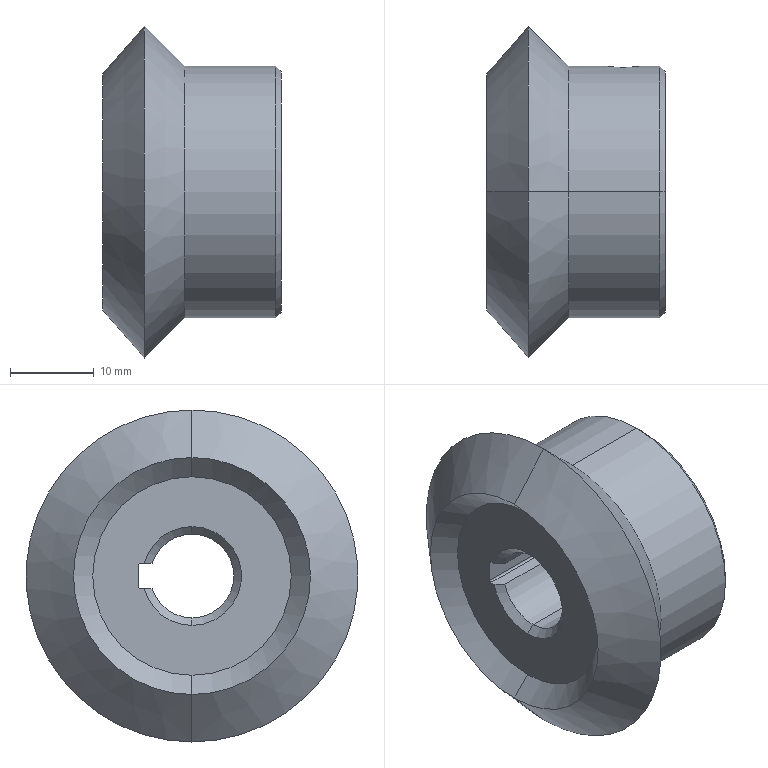Part | SolidWorks | features RefAxis 12, 3DProfileFeature 4, RevCut 2, ICE 1, Revolution 1 | 1 solid | 35 faces | box 21.26 x 39.62 x 39.62 mm | volume 14366 mm3 | cone 16 | cylinder 11 | plane 8 | commonest cylinder face diameters 0.4 x4 10 x3 3.242 x2 30 x2
STEP:
#1=CARTESIAN_POINT('',(-5.615,4.77,-1.5));
#2=VERTEX_POINT('',#1);
#3=CARTESIAN_POINT('',(-5.,4.73,-1.621));
#4=VERTEX_POINT('',#3);
#5=CARTESIAN_POINT('',(-5.615,4.77,-1.5));
#6=CARTESIAN_POINT('',(-5.518,4.757,-1.54));
#7=CARTESIAN_POINT('',(-5.418,4.747,-1.57));
#8=CARTESIAN_POINT('',(-5.211,4.734,-1.611));
#9=CARTESIAN_POINT('',(-5.105,4.73,-1.621));
#10=CARTESIAN_POINT('',(-5.,4.73,-1.621));
#11=B_SPLINE_CURVE_WITH_KNOTS('',3,(#5,#6,#7,#8,#9,#10),.UNSPECIFIED.,.F.,.F.,(4,2,4),(0.004473,0.004788,0.005103),.UNSPECIFIED.);
#12=EDGE_CURVE('',#2,#4,#11,.T.);
#13=ORIENTED_EDGE('',*,*,#12,.T.);
#14=CARTESIAN_POINT('',(-5.,14.621,-1.621));
#15=VERTEX_POINT('',#14);
#16=CARTESIAN_POINT('',(-5.,4.583,-1.621));
#17=DIRECTION('',(0.,1.,0.));
#18=VECTOR('',#17,1000.);
#19=LINE('',#16,#18);
#20=EDGE_CURVE('',#4,#15,#19,.T.);
#21=ORIENTED_EDGE('',*,*,#20,.T.);
#22=CARTESIAN_POINT('',(-5.,14.621,1.621));
#23=VERTEX_POINT('',#22);
#24=CARTESIAN_POINT('',(-5.,14.621,0.));
#25=DIRECTION('',(0.,1.,0.));
#26=DIRECTION('',(0.,0.,1.));
#27=AXIS2_PLACEMENT_3D('',#24,#25,#26);
#28=CIRCLE('',#27,1.621);
#29=EDGE_CURVE('',#15,#23,#28,.T.);
#30=ORIENTED_EDGE('',*,*,#29,.T.);
#31=CARTESIAN_POINT('',(-5.,4.73,1.621));
#32=VERTEX_POINT('',#31);
#33=CARTESIAN_POINT('',(-5.,4.583,1.621));
#34=DIRECTION('',(0.,1.,0.));
#35=VECTOR('',#34,1000.);
#36=LINE('',#33,#35);
#37=EDGE_CURVE('',#32,#23,#36,.T.);
#38=ORIENTED_EDGE('',*,*,#37,.F.);
#39=CARTESIAN_POINT('',(-5.615,4.77,1.5));
#40=VERTEX_POINT('',#39);
#41=CARTESIAN_POINT('',(-5.,4.73,1.621));
#42=CARTESIAN_POINT('',(-5.106,4.73,1.621));
#43=CARTESIAN_POINT('',(-5.211,4.734,1.611));
#44=CARTESIAN_POINT('',(-5.416,4.747,1.57));
#45=CARTESIAN_POINT('',(-5.518,4.757,1.54));
#46=CARTESIAN_POINT('',(-5.615,4.77,1.5));
#47=B_SPLINE_CURVE_WITH_KNOTS('',3,(#41,#42,#43,#44,#45,#46),.UNSPECIFIED.,.F.,.F.,(4,2,4),(0.,0.0003142,0.0006283),.UNSPECIFIED.);
#48=EDGE_CURVE('',#32,#40,#47,.T.);
#49=ORIENTED_EDGE('',*,*,#48,.T.);
#50=CARTESIAN_POINT('',(-5.615,6.2,1.5));
#51=VERTEX_POINT('',#50);
#52=CARTESIAN_POINT('',(-5.615,4.583,1.5));
#53=DIRECTION('',(0.,-1.,0.));
#54=VECTOR('',#53,1000.);
#55=LINE('',#52,#54);
#56=EDGE_CURVE('',#51,#40,#55,.T.);
#57=ORIENTED_EDGE('',*,*,#56,.F.);
#58=CARTESIAN_POINT('',(-5.968,6.4,1.3));
#59=VERTEX_POINT('',#58);
#60=CARTESIAN_POINT('',(-5.968,6.4,1.3));
#61=CARTESIAN_POINT('',(-5.903,6.4,1.349));
#62=CARTESIAN_POINT('',(-5.836,6.384,1.391));
#63=CARTESIAN_POINT('',(-5.736,6.34,1.445));
#64=CARTESIAN_POINT('',(-5.704,6.322,1.461));
#65=CARTESIAN_POINT('',(-5.659,6.286,1.481));
#66=CARTESIAN_POINT('',(-5.645,6.272,1.487));
#67=CARTESIAN_POINT('',(-5.623,6.24,1.497));
#68=CARTESIAN_POINT('',(-5.615,6.221,1.5));
#69=CARTESIAN_POINT('',(-5.615,6.2,1.5));
#70=B_SPLINE_CURVE_WITH_KNOTS('',3,(#60,#61,#62,#63,#64,#65,#66,#67,#68,#69),.UNSPECIFIED.,.F.,.F.,(4,2,2,2,4),(0.,0.0002404,0.0003606,0.0004207,0.0004807),.UNSPECIFIED.);
#71=EDGE_CURVE('',#59,#51,#70,.T.);
#72=ORIENTED_EDGE('',*,*,#71,.F.);
#73=CARTESIAN_POINT('',(-5.968,6.4,-1.3));
#74=VERTEX_POINT('',#73);
#75=CARTESIAN_POINT('',(-5.,6.4,0.));
#76=DIRECTION('',(0.,1.,0.));
#77=DIRECTION('',(0.,0.,1.));
#78=AXIS2_PLACEMENT_3D('',#75,#76,#77);
#79=CIRCLE('',#78,1.621);
#80=EDGE_CURVE('',#74,#59,#79,.T.);
#81=ORIENTED_EDGE('',*,*,#80,.F.);
#82=CARTESIAN_POINT('',(-5.615,6.2,-1.5));
#83=VERTEX_POINT('',#82);
#84=CARTESIAN_POINT('',(-5.615,6.2,-1.5));
#85=CARTESIAN_POINT('',(-5.615,6.221,-1.5));
#86=CARTESIAN_POINT('',(-5.623,6.24,-1.497));
#87=CARTESIAN_POINT('',(-5.645,6.273,-1.487));
#88=CARTESIAN_POINT('',(-5.659,6.286,-1.481));
#89=CARTESIAN_POINT('',(-5.704,6.322,-1.461));
#90=CARTESIAN_POINT('',(-5.736,6.34,-1.445));
#91=CARTESIAN_POINT('',(-5.836,6.384,-1.391));
#92=CARTESIAN_POINT('',(-5.903,6.4,-1.349));
#93=CARTESIAN_POINT('',(-5.968,6.4,-1.3));
#94=B_SPLINE_CURVE_WITH_KNOTS('',3,(#84,#85,#86,#87,#88,#89,#90,#91,#92,#93),.UNSPECIFIED.,.F.,.F.,(4,2,2,2,4),(0.,0.00006084,0.0001217,0.0002434,0.0004867),.UNSPECIFIED.);
#95=EDGE_CURVE('',#83,#74,#94,.T.);
#96=ORIENTED_EDGE('',*,*,#95,.F.);
#97=CARTESIAN_POINT('',(-5.615,4.583,-1.5));
#98=DIRECTION('',(0.,1.,0.));
#99=VECTOR('',#98,1000.);
#100=LINE('',#97,#99);
#101=EDGE_CURVE('',#2,#83,#100,.T.);
#102=ORIENTED_EDGE('',*,*,#101,.F.);
#103=EDGE_LOOP('',(#13,#21,#30,#38,#49,#57,#72,#81,#96,#102));
#104=FACE_OUTER_BOUND('',#103,.T.);
#105=CARTESIAN_POINT('',(-5.,4.583,0.));
#106=DIRECTION('',(0.,1.,0.));
#107=DIRECTION('',(0.,0.,1.));
#108=AXIS2_PLACEMENT_3D('',#105,#106,#107);
#109=CYLINDRICAL_SURFACE('',#108,1.621);
#110=ADVANCED_FACE('',(#104),#109,.F.);
#111=ORIENTED_EDGE('',*,*,#29,.F.);
#112=CARTESIAN_POINT('',(-5.,14.882,-1.882));
#113=VERTEX_POINT('',#112);
#114=CARTESIAN_POINT('',(-5.,14.621,-1.621));
#115=DIRECTION('',(0.,0.7071,-0.7071));
#116=VECTOR('',#115,1000.);
#117=LINE('',#114,#116);
#118=EDGE_CURVE('',#15,#113,#117,.T.);
#119=ORIENTED_EDGE('',*,*,#118,.T.);
#120=CARTESIAN_POINT('',(-5.,14.882,1.882));
#121=VERTEX_POINT('',#120);
#122=CARTESIAN_POINT('',(-5.,14.882,-1.882));
#123=CARTESIAN_POINT('',(-5.127,14.882,-1.882));
#124=CARTESIAN_POINT('',(-5.255,14.883,-1.87));
#125=CARTESIAN_POINT('',(-5.505,14.889,-1.824));
#126=CARTESIAN_POINT('',(-5.627,14.893,-1.791));
#127=CARTESIAN_POINT('',(-5.864,14.903,-1.701));
#128=CARTESIAN_POINT('',(-5.98,14.91,-1.644));
#129=CARTESIAN_POINT('',(-6.196,14.924,-1.512));
#130=CARTESIAN_POINT('',(-6.298,14.931,-1.436));
#131=CARTESIAN_POINT('',(-6.487,14.947,-1.263));
#132=CARTESIAN_POINT('',(-6.572,14.955,-1.169));
#133=CARTESIAN_POINT('',(-6.722,14.969,-0.9645));
#134=CARTESIAN_POINT('',(-6.787,14.976,-0.8532));
#135=CARTESIAN_POINT('',(-6.944,14.993,-0.5079));
#136=CARTESIAN_POINT('',(-7.,15.,-0.2529));
#137=CARTESIAN_POINT('',(-7.,15.,0.1265));
#138=CARTESIAN_POINT('',(-6.986,14.998,0.2546));
#139=CARTESIAN_POINT('',(-6.932,14.992,0.5033));
#140=CARTESIAN_POINT('',(-6.891,14.987,0.6233));
#141=CARTESIAN_POINT('',(-6.786,14.976,0.8548));
#142=CARTESIAN_POINT('',(-6.721,14.969,0.9657));
#143=CARTESIAN_POINT('',(-6.571,14.955,1.17));
#144=CARTESIAN_POINT('',(-6.486,14.947,1.265));
#145=CARTESIAN_POINT('',(-6.297,14.931,1.436));
#146=CARTESIAN_POINT('',(-6.196,14.924,1.512));
#147=CARTESIAN_POINT('',(-5.98,14.91,1.644));
#148=CARTESIAN_POINT('',(-5.864,14.903,1.701));
#149=CARTESIAN_POINT('',(-5.627,14.893,1.791));
#150=CARTESIAN_POINT('',(-5.505,14.889,1.824));
#151=CARTESIAN_POINT('',(-5.255,14.883,1.87));
#152=CARTESIAN_POINT('',(-5.127,14.882,1.882));
#153=CARTESIAN_POINT('',(-5.,14.882,1.882));
#154=B_SPLINE_CURVE_WITH_KNOTS('',3,(#122,#123,#124,#125,#126,#127,#128,#129,#130,#131,#132,#133,#134,#135,#136,#137,#138,#139,#140,#141,#142,#143,#144,#145,#146,#147,#148,#149,#150,#151,#152,#153),.UNSPECIFIED.,.F.,.F.,(4,2,2,2,2,2,2,2,2,2,2,2,2,2,2,4),(0.01068,0.01106,0.01145,0.01183,0.01221,0.01259,0.01297,0.01373,0.01411,0.01449,0.01487,0.01525,0.01563,0.01601,0.01639,0.01677),.UNSPECIFIED.);
#155=EDGE_CURVE('',#113,#121,#154,.T.);
#156=ORIENTED_EDGE('',*,*,#155,.T.);
#157=CARTESIAN_POINT('',(-5.,14.621,1.621));
#158=DIRECTION('',(0.,0.7071,0.7071));
#159=VECTOR('',#158,1000.);
#160=LINE('',#157,#159);
#161=EDGE_CURVE('',#23,#121,#160,.T.);
#162=ORIENTED_EDGE('',*,*,#161,.F.);
#163=EDGE_LOOP('',(#111,#119,#156,#162));
#164=FACE_OUTER_BOUND('',#163,.T.);
#165=CARTESIAN_POINT('',(-5.,14.621,0.));
#166=DIRECTION('',(0.,1.,0.));
#167=DIRECTION('',(0.,0.,1.));
#168=AXIS2_PLACEMENT_3D('',#165,#166,#167);
#169=CONICAL_SURFACE('',#168,1.621,0.7854);
#170=ADVANCED_FACE('',(#164),#169,.F.);
#171=CARTESIAN_POINT('',(-0.9,0.,-5.));
#172=VERTEX_POINT('',#171);
#173=CARTESIAN_POINT('',(-0.9,0.,5.));
#174=VERTEX_POINT('',#173);
#175=CARTESIAN_POINT('',(-0.9,0.,0.));
#176=DIRECTION('',(-1.,0.,0.));
#177=DIRECTION('',(0.,0.,1.));
#178=AXIS2_PLACEMENT_3D('',#175,#176,#177);
#179=CIRCLE('',#178,5.);
#180=EDGE_CURVE('',#172,#174,#179,.T.);
#181=ORIENTED_EDGE('',*,*,#180,.T.);
#182=CARTESIAN_POINT('',(0.,0.,5.9));
#183=VERTEX_POINT('',#182);
#184=CARTESIAN_POINT('',(0.,0.,5.9));
#185=DIRECTION('',(0.7071,0.,0.7071));
#186=VECTOR('',#185,1000.);
#187=LINE('',#184,#186);
#188=EDGE_CURVE('',#174,#183,#187,.T.);
#189=ORIENTED_EDGE('',*,*,#188,.T.);
#190=CARTESIAN_POINT('',(0.,0.,-5.9));
#191=VERTEX_POINT('',#190);
#192=CARTESIAN_POINT('',(0.,0.,0.));
#193=DIRECTION('',(-1.,0.,0.));
#194=DIRECTION('',(0.,0.,1.));
#195=AXIS2_PLACEMENT_3D('',#192,#193,#194);
#196=CIRCLE('',#195,5.9);
#197=EDGE_CURVE('',#191,#183,#196,.T.);
#198=ORIENTED_EDGE('',*,*,#197,.F.);
#199=CARTESIAN_POINT('',(0.,0.,-5.9));
#200=DIRECTION('',(0.7071,0.,-0.7071));
#201=VECTOR('',#200,1000.);
#202=LINE('',#199,#201);
#203=EDGE_CURVE('',#172,#191,#202,.T.);
#204=ORIENTED_EDGE('',*,*,#203,.F.);
#205=EDGE_LOOP('',(#181,#189,#198,#204));
#206=FACE_OUTER_BOUND('',#205,.T.);
#207=CARTESIAN_POINT('',(0.,0.,0.));
#208=DIRECTION('',(1.,0.,0.));
#209=DIRECTION('',(0.,0.,-1.));
#210=AXIS2_PLACEMENT_3D('',#207,#208,#209);
#211=CONICAL_SURFACE('',#210,5.9,0.7854);
#212=ADVANCED_FACE('',(#206),#211,.F.);
#213=CARTESIAN_POINT('',(-0.9,4.77,-1.5));
#214=VERTEX_POINT('',#213);
#215=CARTESIAN_POINT('',(-0.9,0.,0.));
#216=DIRECTION('',(-1.,0.,0.));
#217=DIRECTION('',(0.,0.,1.));
#218=AXIS2_PLACEMENT_3D('',#215,#216,#217);
#219=CIRCLE('',#218,5.);
#220=EDGE_CURVE('',#214,#172,#219,.T.);
#221=ORIENTED_EDGE('',*,*,#220,.T.);
#222=ORIENTED_EDGE('',*,*,#203,.T.);
#223=CARTESIAN_POINT('',(0.,5.706,-1.5));
#224=VERTEX_POINT('',#223);
#225=CARTESIAN_POINT('',(0.,0.,0.));
#226=DIRECTION('',(-1.,0.,0.));
#227=DIRECTION('',(0.,0.,1.));
#228=AXIS2_PLACEMENT_3D('',#225,#226,#227);
#229=CIRCLE('',#228,5.9);
#230=EDGE_CURVE('',#224,#191,#229,.T.);
#231=ORIENTED_EDGE('',*,*,#230,.F.);
#232=CARTESIAN_POINT('',(-0.9,4.77,-1.5));
#233=CARTESIAN_POINT('',(-0.6012,5.083,-1.5));
#234=CARTESIAN_POINT('',(-0.301,5.395,-1.5));
#235=CARTESIAN_POINT('',(0.,5.706,-1.5));
#236=B_SPLINE_CURVE_WITH_KNOTS('',3,(#232,#233,#234,#235),.UNSPECIFIED.,.F.,.F.,(4,4),(0.01043,0.01174),.UNSPECIFIED.);
#237=EDGE_CURVE('',#214,#224,#236,.T.);
#238=ORIENTED_EDGE('',*,*,#237,.F.);
#239=EDGE_LOOP('',(#221,#222,#231,#238));
#240=FACE_OUTER_BOUND('',#239,.T.);
#241=CARTESIAN_POINT('',(0.,0.,0.));
#242=DIRECTION('',(1.,0.,0.));
#243=DIRECTION('',(0.,0.,-1.));
#244=AXIS2_PLACEMENT_3D('',#241,#242,#243);
#245=CONICAL_SURFACE('',#244,5.9,0.7854);
#246=ADVANCED_FACE('',(#240),#245,.F.);
#247=CARTESIAN_POINT('',(-18.1,0.,-5.));
#248=VERTEX_POINT('',#247);
#249=CARTESIAN_POINT('',(-18.1,0.,5.));
#250=VERTEX_POINT('',#249);
#251=CARTESIAN_POINT('',(-18.1,0.,0.));
#252=DIRECTION('',(-1.,0.,0.));
#253=DIRECTION('',(0.,0.,1.));
#254=AXIS2_PLACEMENT_3D('',#251,#252,#253);
#255=CIRCLE('',#254,5.);
#256=EDGE_CURVE('',#248,#250,#255,.T.);
#257=ORIENTED_EDGE('',*,*,#256,.F.);
#258=CARTESIAN_POINT('',(-19.,0.,-5.9));
#259=VERTEX_POINT('',#258);
#260=CARTESIAN_POINT('',(-18.1,0.,-5.));
#261=DIRECTION('',(-0.7071,0.,-0.7071));
#262=VECTOR('',#261,1000.);
#263=LINE('',#260,#262);
#264=EDGE_CURVE('',#248,#259,#263,.T.);
#265=ORIENTED_EDGE('',*,*,#264,.T.);
#266=CARTESIAN_POINT('',(-19.,0.,5.9));
#267=VERTEX_POINT('',#266);
#268=CARTESIAN_POINT('',(-19.,0.,0.));
#269=DIRECTION('',(-1.,0.,0.));
#270=DIRECTION('',(0.,0.,1.));
#271=AXIS2_PLACEMENT_3D('',#268,#269,#270);
#272=CIRCLE('',#271,5.9);
#273=EDGE_CURVE('',#259,#267,#272,.T.);
#274=ORIENTED_EDGE('',*,*,#273,.T.);
#275=CARTESIAN_POINT('',(-18.1,0.,5.));
#276=DIRECTION('',(-0.7071,0.,0.7071));
#277=VECTOR('',#276,1000.);
#278=LINE('',#275,#277);
#279=EDGE_CURVE('',#250,#267,#278,.T.);
#280=ORIENTED_EDGE('',*,*,#279,.F.);
#281=EDGE_LOOP('',(#257,#265,#274,#280));
#282=FACE_OUTER_BOUND('',#281,.T.);
#283=CARTESIAN_POINT('',(-18.1,0.,0.));
#284=DIRECTION('',(-1.,0.,0.));
#285=DIRECTION('',(0.,0.,1.));
#286=AXIS2_PLACEMENT_3D('',#283,#284,#285);
#287=CONICAL_SURFACE('',#286,5.,0.7854);
#288=ADVANCED_FACE('',(#282),#287,.F.);
#289=CARTESIAN_POINT('',(-18.1,4.77,1.5));
#290=VERTEX_POINT('',#289);
#291=CARTESIAN_POINT('',(-18.1,0.,0.));
#292=DIRECTION('',(-1.,0.,0.));
#293=DIRECTION('',(0.,0.,1.));
#294=AXIS2_PLACEMENT_3D('',#291,#292,#293);
#295=CIRCLE('',#294,5.);
#296=EDGE_CURVE('',#250,#290,#295,.T.);
#297=ORIENTED_EDGE('',*,*,#296,.F.);
#298=ORIENTED_EDGE('',*,*,#279,.T.);
#299=CARTESIAN_POINT('',(-19.,5.706,1.5));
#300=VERTEX_POINT('',#299);
#301=CARTESIAN_POINT('',(-19.,0.,0.));
#302=DIRECTION('',(-1.,0.,0.));
#303=DIRECTION('',(0.,0.,1.));
#304=AXIS2_PLACEMENT_3D('',#301,#302,#303);
#305=CIRCLE('',#304,5.9);
#306=EDGE_CURVE('',#267,#300,#305,.T.);
#307=ORIENTED_EDGE('',*,*,#306,.T.);
#308=CARTESIAN_POINT('',(-18.1,4.77,1.5));
#309=CARTESIAN_POINT('',(-18.399,5.083,1.5));
#310=CARTESIAN_POINT('',(-18.699,5.395,1.5));
#311=CARTESIAN_POINT('',(-19.,5.706,1.5));
#312=B_SPLINE_CURVE_WITH_KNOTS('',3,(#308,#309,#310,#311),.UNSPECIFIED.,.F.,.F.,(4,4),(0.01043,0.01174),.UNSPECIFIED.);
#313=EDGE_CURVE('',#290,#300,#312,.T.);
#314=ORIENTED_EDGE('',*,*,#313,.F.);
#315=EDGE_LOOP('',(#297,#298,#307,#314));
#316=FACE_OUTER_BOUND('',#315,.T.);
#317=CARTESIAN_POINT('',(-18.1,0.,0.));
#318=DIRECTION('',(-1.,0.,0.));
#319=DIRECTION('',(0.,0.,1.));
#320=AXIS2_PLACEMENT_3D('',#317,#318,#319);
#321=CONICAL_SURFACE('',#320,5.,0.7854);
#322=ADVANCED_FACE('',(#316),#321,.F.);
#323=CARTESIAN_POINT('',(-19.,0.,-11.85));
#324=VERTEX_POINT('',#323);
#325=CARTESIAN_POINT('',(-19.,0.,11.85));
#326=VERTEX_POINT('',#325);
#327=CARTESIAN_POINT('',(-19.,0.,0.));
#328=DIRECTION('',(-1.,0.,0.));
#329=DIRECTION('',(0.,0.,1.));
#330=AXIS2_PLACEMENT_3D('',#327,#328,#329);
#331=CIRCLE('',#330,11.85);
#332=EDGE_CURVE('',#324,#326,#331,.T.);
#333=ORIENTED_EDGE('',*,*,#332,.F.);
#334=CARTESIAN_POINT('',(-21.26,0.,-14.146));
#335=VERTEX_POINT('',#334);
#336=CARTESIAN_POINT('',(-21.26,0.,-14.146));
#337=DIRECTION('',(-0.7015,0.,-0.7126));
#338=VECTOR('',#337,1000.);
#339=LINE('',#336,#338);
#340=EDGE_CURVE('',#324,#335,#339,.T.);
#341=ORIENTED_EDGE('',*,*,#340,.T.);
#342=CARTESIAN_POINT('',(-21.26,0.,14.146));
#343=VERTEX_POINT('',#342);
#344=CARTESIAN_POINT('',(-21.26,0.,0.));
#345=DIRECTION('',(-1.,0.,0.));
#346=DIRECTION('',(0.,0.,1.));
#347=AXIS2_PLACEMENT_3D('',#344,#345,#346);
#348=CIRCLE('',#347,14.146);
#349=EDGE_CURVE('',#335,#343,#348,.T.);
#350=ORIENTED_EDGE('',*,*,#349,.T.);
#351=CARTESIAN_POINT('',(-21.26,0.,14.146));
#352=DIRECTION('',(-0.7015,0.,0.7126));
#353=VECTOR('',#352,1000.);
#354=LINE('',#351,#353);
#355=EDGE_CURVE('',#326,#343,#354,.T.);
#356=ORIENTED_EDGE('',*,*,#355,.F.);
#357=EDGE_LOOP('',(#333,#341,#350,#356));
#358=FACE_OUTER_BOUND('',#357,.T.);
#359=CARTESIAN_POINT('',(-21.26,0.,0.));
#360=DIRECTION('',(-1.,0.,0.));
#361=DIRECTION('',(0.,0.,1.));
#362=AXIS2_PLACEMENT_3D('',#359,#360,#361);
#363=CONICAL_SURFACE('',#362,14.146,0.7932);
#364=ADVANCED_FACE('',(#358),#363,.F.);
#365=CARTESIAN_POINT('',(0.,0.,14.364));
#366=VERTEX_POINT('',#365);
#367=CARTESIAN_POINT('',(0.,0.,-14.364));
#368=VERTEX_POINT('',#367);
#369=CARTESIAN_POINT('',(0.,0.,0.));
#370=DIRECTION('',(-1.,0.,0.));
#371=DIRECTION('',(0.,0.,1.));
#372=AXIS2_PLACEMENT_3D('',#369,#370,#371);
#373=CIRCLE('',#372,14.364);
#374=EDGE_CURVE('',#366,#368,#373,.T.);
#375=ORIENTED_EDGE('',*,*,#374,.T.);
#376=CARTESIAN_POINT('',(-0.6364,0.,-15.));
#377=VERTEX_POINT('',#376);
#378=CARTESIAN_POINT('',(0.,0.,-14.364));
#379=DIRECTION('',(-0.7071,0.,-0.7071));
#380=VECTOR('',#379,1000.);
#381=LINE('',#378,#380);
#382=EDGE_CURVE('',#368,#377,#381,.T.);
#383=ORIENTED_EDGE('',*,*,#382,.T.);
#384=CARTESIAN_POINT('',(-0.6364,0.,15.));
#385=VERTEX_POINT('',#384);
#386=CARTESIAN_POINT('',(-0.6364,0.,0.));
#387=DIRECTION('',(-1.,0.,0.));
#388=DIRECTION('',(0.,0.,1.));
#389=AXIS2_PLACEMENT_3D('',#386,#387,#388);
#390=CIRCLE('',#389,15.);
#391=EDGE_CURVE('',#385,#377,#390,.T.);
#392=ORIENTED_EDGE('',*,*,#391,.F.);
#393=CARTESIAN_POINT('',(0.,0.,14.364));
#394=DIRECTION('',(-0.7071,0.,0.7071));
#395=VECTOR('',#394,1000.);
#396=LINE('',#393,#395);
#397=EDGE_CURVE('',#366,#385,#396,.T.);
#398=ORIENTED_EDGE('',*,*,#397,.F.);
#399=EDGE_LOOP('',(#375,#383,#392,#398));
#400=FACE_OUTER_BOUND('',#399,.T.);
#401=CARTESIAN_POINT('',(0.,0.,0.));
#402=DIRECTION('',(-1.,0.,0.));
#403=DIRECTION('',(0.,0.,1.));
#404=AXIS2_PLACEMENT_3D('',#401,#402,#403);
#405=CONICAL_SURFACE('',#404,14.364,0.7854);
#406=ADVANCED_FACE('',(#400),#405,.T.);
#407=CARTESIAN_POINT('',(-11.5,0.,15.));
#408=VERTEX_POINT('',#407);
#409=CARTESIAN_POINT('',(-11.5,0.,-15.));
#410=VERTEX_POINT('',#409);
#411=CARTESIAN_POINT('',(-11.5,0.,0.));
#412=DIRECTION('',(-1.,0.,0.));
#413=DIRECTION('',(0.,0.,1.));
#414=AXIS2_PLACEMENT_3D('',#411,#412,#413);
#415=CIRCLE('',#414,15.);
#416=EDGE_CURVE('',#408,#410,#415,.T.);
#417=ORIENTED_EDGE('',*,*,#416,.T.);
#418=CARTESIAN_POINT('',(-16.31,0.,-19.81));
#419=VERTEX_POINT('',#418);
#420=CARTESIAN_POINT('',(-11.5,0.,-15.));
#421=DIRECTION('',(-0.7071,0.,-0.7071));
#422=VECTOR('',#421,1000.);
#423=LINE('',#420,#422);
#424=EDGE_CURVE('',#410,#419,#423,.T.);
#425=ORIENTED_EDGE('',*,*,#424,.T.);
#426=CARTESIAN_POINT('',(-16.31,0.,19.81));
#427=VERTEX_POINT('',#426);
#428=CARTESIAN_POINT('',(-16.31,0.,0.));
#429=DIRECTION('',(-1.,0.,0.));
#430=DIRECTION('',(0.,0.,1.));
#431=AXIS2_PLACEMENT_3D('',#428,#429,#430);
#432=CIRCLE('',#431,19.81);
#433=EDGE_CURVE('',#427,#419,#432,.T.);
#434=ORIENTED_EDGE('',*,*,#433,.F.);
#435=CARTESIAN_POINT('',(-11.5,0.,15.));
#436=DIRECTION('',(-0.7071,0.,0.7071));
#437=VECTOR('',#436,1000.);
#438=LINE('',#435,#437);
#439=EDGE_CURVE('',#408,#427,#438,.T.);
#440=ORIENTED_EDGE('',*,*,#439,.F.);
#441=EDGE_LOOP('',(#417,#425,#434,#440));
#442=FACE_OUTER_BOUND('',#441,.T.);
#443=CARTESIAN_POINT('',(-11.5,0.,0.));
#444=DIRECTION('',(-1.,0.,0.));
#445=DIRECTION('',(0.,0.,1.));
#446=AXIS2_PLACEMENT_3D('',#443,#444,#445);
#447=CONICAL_SURFACE('',#446,15.,0.7854);
#448=ADVANCED_FACE('',(#442),#447,.T.);
#449=CARTESIAN_POINT('',(-21.26,0.,0.));
#450=DIRECTION('',(-1.,0.,0.));
#451=DIRECTION('',(0.,0.,1.));
#452=AXIS2_PLACEMENT_3D('',#449,#450,#451);
#453=CIRCLE('',#452,14.146);
#454=EDGE_CURVE('',#343,#335,#453,.T.);
#455=ORIENTED_EDGE('',*,*,#454,.F.);
#456=CARTESIAN_POINT('',(-16.31,0.,19.81));
#457=DIRECTION('',(0.658,0.,0.753));
#458=VECTOR('',#457,1000.);
#459=LINE('',#456,#458);
#460=EDGE_CURVE('',#343,#427,#459,.T.);
#461=ORIENTED_EDGE('',*,*,#460,.T.);
#462=ORIENTED_EDGE('',*,*,#433,.T.);
#463=CARTESIAN_POINT('',(-16.31,0.,-19.81));
#464=DIRECTION('',(0.658,0.,-0.753));
#465=VECTOR('',#464,1000.);
#466=LINE('',#463,#465);
#467=EDGE_CURVE('',#335,#419,#466,.T.);
#468=ORIENTED_EDGE('',*,*,#467,.F.);
#469=EDGE_LOOP('',(#455,#461,#462,#468));
#470=FACE_OUTER_BOUND('',#469,.T.);
#471=CARTESIAN_POINT('',(-16.31,0.,0.));
#472=DIRECTION('',(1.,0.,0.));
#473=DIRECTION('',(0.,0.,-1.));
#474=AXIS2_PLACEMENT_3D('',#471,#472,#473);
#475=CONICAL_SURFACE('',#474,19.81,0.8526);
#476=ADVANCED_FACE('',(#470),#475,.T.);
#477=ORIENTED_EDGE('',*,*,#180,.F.);
#478=CARTESIAN_POINT('',(0.,0.,-5.));
#479=DIRECTION('',(-1.,0.,0.));
#480=VECTOR('',#479,1000.);
#481=LINE('',#478,#480);
#482=EDGE_CURVE('',#172,#248,#481,.T.);
#483=ORIENTED_EDGE('',*,*,#482,.T.);
#484=ORIENTED_EDGE('',*,*,#256,.T.);
#485=CARTESIAN_POINT('',(0.,0.,5.));
#486=DIRECTION('',(-1.,0.,0.));
#487=VECTOR('',#486,1000.);
#488=LINE('',#485,#487);
#489=EDGE_CURVE('',#174,#250,#488,.T.);
#490=ORIENTED_EDGE('',*,*,#489,.F.);
#491=EDGE_LOOP('',(#477,#483,#484,#490));
#492=FACE_OUTER_BOUND('',#491,.T.);
#493=CARTESIAN_POINT('',(0.,0.,0.));
#494=DIRECTION('',(-1.,0.,0.));
#495=DIRECTION('',(0.,0.,1.));
#496=AXIS2_PLACEMENT_3D('',#493,#494,#495);
#497=CYLINDRICAL_SURFACE('',#496,5.);
#498=ADVANCED_FACE('',(#492),#497,.F.);
#499=CARTESIAN_POINT('',(-0.9,4.77,1.5));
#500=VERTEX_POINT('',#499);
#501=CARTESIAN_POINT('',(-0.9,0.,0.));
#502=DIRECTION('',(-1.,0.,0.));
#503=DIRECTION('',(0.,0.,1.));
#504=AXIS2_PLACEMENT_3D('',#501,#502,#503);
#505=CIRCLE('',#504,5.);
#506=EDGE_CURVE('',#174,#500,#505,.T.);
#507=ORIENTED_EDGE('',*,*,#506,.F.);
#508=ORIENTED_EDGE('',*,*,#489,.T.);
#509=ORIENTED_EDGE('',*,*,#296,.T.);
#510=CARTESIAN_POINT('',(0.,4.77,1.5));
#511=DIRECTION('',(1.,0.,0.));
#512=VECTOR('',#511,1000.);
#513=LINE('',#510,#512);
#514=EDGE_CURVE('',#290,#40,#513,.T.);
#515=ORIENTED_EDGE('',*,*,#514,.T.);
#516=ORIENTED_EDGE('',*,*,#48,.F.);
#517=CARTESIAN_POINT('',(-4.385,4.77,1.5));
#518=VERTEX_POINT('',#517);
#519=CARTESIAN_POINT('',(-4.385,4.77,1.5));
#520=CARTESIAN_POINT('',(-4.482,4.757,1.54));
#521=CARTESIAN_POINT('',(-4.584,4.747,1.57));
#522=CARTESIAN_POINT('',(-4.789,4.734,1.611));
#523=CARTESIAN_POINT('',(-4.894,4.73,1.621));
#524=CARTESIAN_POINT('',(-5.,4.73,1.621));
#525=B_SPLINE_CURVE_WITH_KNOTS('',3,(#519,#520,#521,#522,#523,#524),.UNSPECIFIED.,.F.,.F.,(4,2,4),(0.009576,0.00989,0.0102),.UNSPECIFIED.);
#526=EDGE_CURVE('',#518,#32,#525,.T.);
#527=ORIENTED_EDGE('',*,*,#526,.F.);
#528=CARTESIAN_POINT('',(0.,4.77,1.5));
#529=DIRECTION('',(1.,0.,0.));
#530=VECTOR('',#529,1000.);
#531=LINE('',#528,#530);
#532=EDGE_CURVE('',#518,#500,#531,.T.);
#533=ORIENTED_EDGE('',*,*,#532,.T.);
#534=EDGE_LOOP('',(#507,#508,#509,#515,#516,#527,#533));
#535=FACE_OUTER_BOUND('',#534,.T.);
#536=CARTESIAN_POINT('',(0.,0.,0.));
#537=DIRECTION('',(-1.,0.,0.));
#538=DIRECTION('',(0.,0.,1.));
#539=AXIS2_PLACEMENT_3D('',#536,#537,#538);
#540=CYLINDRICAL_SURFACE('',#539,5.);
#541=ADVANCED_FACE('',(#535),#540,.F.);
#542=CARTESIAN_POINT('',(-5.,14.882,1.882));
#543=CARTESIAN_POINT('',(-4.747,14.882,1.882));
#544=CARTESIAN_POINT('',(-4.491,14.888,1.835));
#545=CARTESIAN_POINT('',(-4.018,14.909,1.656));
#546=CARTESIAN_POINT('',(-3.796,14.924,1.521));
#547=CARTESIAN_POINT('',(-3.423,14.954,1.181));
#548=CARTESIAN_POINT('',(-3.268,14.97,0.9719));
#549=CARTESIAN_POINT('',(-3.11,14.987,0.627));
#550=CARTESIAN_POINT('',(-3.069,14.992,0.5042));
#551=CARTESIAN_POINT('',(-3.014,14.998,0.2562));
#552=CARTESIAN_POINT('',(-3.,15.,0.1305));
#553=CARTESIAN_POINT('',(-3.,15.,-0.2521));
#554=CARTESIAN_POINT('',(-3.055,14.993,-0.5062));
#555=CARTESIAN_POINT('',(-3.214,14.976,-0.8546));
#556=CARTESIAN_POINT('',(-3.278,14.969,-0.9637));
#557=CARTESIAN_POINT('',(-3.428,14.955,-1.169));
#558=CARTESIAN_POINT('',(-3.514,14.947,-1.265));
#559=CARTESIAN_POINT('',(-3.795,14.924,-1.521));
#560=CARTESIAN_POINT('',(-4.017,14.909,-1.656));
#561=CARTESIAN_POINT('',(-4.372,14.893,-1.79));
#562=CARTESIAN_POINT('',(-4.496,14.889,-1.825));
#563=CARTESIAN_POINT('',(-4.747,14.883,-1.87));
#564=CARTESIAN_POINT('',(-4.873,14.882,-1.882));
#565=CARTESIAN_POINT('',(-5.,14.882,-1.882));
#566=B_SPLINE_CURVE_WITH_KNOTS('',3,(#542,#543,#544,#545,#546,#547,#548,#549,#550,#551,#552,#553,#554,#555,#556,#557,#558,#559,#560,#561,#562,#563,#564,#565),.UNSPECIFIED.,.F.,.F.,(4,2,2,2,2,2,2,2,2,2,2,4),(0.004592,0.005354,0.006115,0.006877,0.007257,0.007638,0.0084,0.00878,0.009161,0.009923,0.0103,0.01068),.UNSPECIFIED.);
#567=EDGE_CURVE('',#121,#113,#566,.T.);
#568=ORIENTED_EDGE('',*,*,#567,.F.);
#569=ORIENTED_EDGE('',*,*,#155,.F.);
#570=EDGE_LOOP('',(#568,#569));
#571=FACE_BOUND('',#570,.T.);
#572=ORIENTED_EDGE('',*,*,#391,.T.);
#573=CARTESIAN_POINT('',(0.,0.,-15.));
#574=DIRECTION('',(-1.,0.,0.));
#575=VECTOR('',#574,1000.);
#576=LINE('',#573,#575);
#577=EDGE_CURVE('',#377,#410,#576,.T.);
#578=ORIENTED_EDGE('',*,*,#577,.T.);
#579=ORIENTED_EDGE('',*,*,#416,.F.);
#580=CARTESIAN_POINT('',(0.,0.,15.));
#581=DIRECTION('',(-1.,0.,0.));
#582=VECTOR('',#581,1000.);
#583=LINE('',#580,#582);
#584=EDGE_CURVE('',#385,#408,#583,.T.);
#585=ORIENTED_EDGE('',*,*,#584,.F.);
#586=EDGE_LOOP('',(#572,#578,#579,#585));
#587=FACE_OUTER_BOUND('',#586,.T.);
#588=CARTESIAN_POINT('',(0.,0.,0.));
#589=DIRECTION('',(-1.,0.,0.));
#590=DIRECTION('',(0.,0.,1.));
#591=AXIS2_PLACEMENT_3D('',#588,#589,#590);
#592=CYLINDRICAL_SURFACE('',#591,15.);
#593=ADVANCED_FACE('',(#571,#587),#592,.T.);
#594=ORIENTED_EDGE('',*,*,#577,.F.);
#595=CARTESIAN_POINT('',(-0.6364,0.,0.));
#596=DIRECTION('',(-1.,0.,0.));
#597=DIRECTION('',(0.,0.,1.));
#598=AXIS2_PLACEMENT_3D('',#595,#596,#597);
#599=CIRCLE('',#598,15.);
#600=EDGE_CURVE('',#377,#385,#599,.T.);
#601=ORIENTED_EDGE('',*,*,#600,.T.);
#602=ORIENTED_EDGE('',*,*,#584,.T.);
#603=CARTESIAN_POINT('',(-11.5,0.,0.));
#604=DIRECTION('',(-1.,0.,0.));
#605=DIRECTION('',(0.,0.,1.));
#606=AXIS2_PLACEMENT_3D('',#603,#604,#605);
#607=CIRCLE('',#606,15.);
#608=EDGE_CURVE('',#410,#408,#607,.T.);
#609=ORIENTED_EDGE('',*,*,#608,.F.);
#610=EDGE_LOOP('',(#594,#601,#602,#609));
#611=FACE_OUTER_BOUND('',#610,.T.);
#612=CARTESIAN_POINT('',(0.,0.,0.));
#613=DIRECTION('',(-1.,0.,0.));
#614=DIRECTION('',(0.,0.,1.));
#615=AXIS2_PLACEMENT_3D('',#612,#613,#614);
#616=CYLINDRICAL_SURFACE('',#615,15.);
#617=ADVANCED_FACE('',(#611),#616,.T.);
#618=ORIENTED_EDGE('',*,*,#482,.F.);
#619=ORIENTED_EDGE('',*,*,#220,.F.);
#620=CARTESIAN_POINT('',(-4.385,4.77,-1.5));
#621=VERTEX_POINT('',#620);
#622=CARTESIAN_POINT('',(0.,4.77,-1.5));
#623=DIRECTION('',(-1.,0.,0.));
#624=VECTOR('',#623,1000.);
#625=LINE('',#622,#624);
#626=EDGE_CURVE('',#214,#621,#625,.T.);
#627=ORIENTED_EDGE('',*,*,#626,.T.);
#628=CARTESIAN_POINT('',(-5.,4.73,-1.621));
#629=CARTESIAN_POINT('',(-4.895,4.73,-1.621));
#630=CARTESIAN_POINT('',(-4.79,4.733,-1.611));
#631=CARTESIAN_POINT('',(-4.582,4.747,-1.57));
#632=CARTESIAN_POINT('',(-4.482,4.757,-1.54));
#633=CARTESIAN_POINT('',(-4.385,4.77,-1.5));
#634=B_SPLINE_CURVE_WITH_KNOTS('',3,(#628,#629,#630,#631,#632,#633),.UNSPECIFIED.,.F.,.F.,(4,2,4),(0.005103,0.005417,0.005732),.UNSPECIFIED.);
#635=EDGE_CURVE('',#4,#621,#634,.T.);
#636=ORIENTED_EDGE('',*,*,#635,.F.);
#637=ORIENTED_EDGE('',*,*,#12,.F.);
#638=CARTESIAN_POINT('',(-18.1,4.77,-1.5));
#639=VERTEX_POINT('',#638);
#640=CARTESIAN_POINT('',(0.,4.77,-1.5));
#641=DIRECTION('',(-1.,0.,0.));
#642=VECTOR('',#641,1000.);
#643=LINE('',#640,#642);
#644=EDGE_CURVE('',#2,#639,#643,.T.);
#645=ORIENTED_EDGE('',*,*,#644,.T.);
#646=CARTESIAN_POINT('',(-18.1,0.,0.));
#647=DIRECTION('',(-1.,0.,0.));
#648=DIRECTION('',(0.,0.,1.));
#649=AXIS2_PLACEMENT_3D('',#646,#647,#648);
#650=CIRCLE('',#649,5.);
#651=EDGE_CURVE('',#639,#248,#650,.T.);
#652=ORIENTED_EDGE('',*,*,#651,.T.);
#653=EDGE_LOOP('',(#618,#619,#627,#636,#637,#645,#652));
#654=FACE_OUTER_BOUND('',#653,.T.);
#655=CARTESIAN_POINT('',(0.,0.,0.));
#656=DIRECTION('',(-1.,0.,0.));
#657=DIRECTION('',(0.,0.,1.));
#658=AXIS2_PLACEMENT_3D('',#655,#656,#657);
#659=CYLINDRICAL_SURFACE('',#658,5.);
#660=ADVANCED_FACE('',(#654),#659,.F.);
#661=ORIENTED_EDGE('',*,*,#374,.F.);
#662=CARTESIAN_POINT('',(0.,0.,0.));
#663=DIRECTION('',(-1.,0.,0.));
#664=DIRECTION('',(0.,0.,1.));
#665=AXIS2_PLACEMENT_3D('',#662,#663,#664);
#666=CIRCLE('',#665,14.364);
#667=EDGE_CURVE('',#368,#366,#666,.T.);
#668=ORIENTED_EDGE('',*,*,#667,.F.);
#669=EDGE_LOOP('',(#661,#668));
#670=FACE_OUTER_BOUND('',#669,.T.);
#671=ORIENTED_EDGE('',*,*,#230,.T.);
#672=ORIENTED_EDGE('',*,*,#197,.T.);
#673=CARTESIAN_POINT('',(0.,5.706,1.5));
#674=VERTEX_POINT('',#673);
#675=CARTESIAN_POINT('',(0.,0.,0.));
#676=DIRECTION('',(-1.,0.,0.));
#677=DIRECTION('',(0.,0.,1.));
#678=AXIS2_PLACEMENT_3D('',#675,#676,#677);
#679=CIRCLE('',#678,5.9);
#680=EDGE_CURVE('',#183,#674,#679,.T.);
#681=ORIENTED_EDGE('',*,*,#680,.T.);
#682=CARTESIAN_POINT('',(0.,6.2,1.5));
#683=VERTEX_POINT('',#682);
#684=CARTESIAN_POINT('',(0.,6.2,1.5));
#685=DIRECTION('',(0.,-1.,0.));
#686=VECTOR('',#685,1000.);
#687=LINE('',#684,#686);
#688=EDGE_CURVE('',#683,#674,#687,.T.);
#689=ORIENTED_EDGE('',*,*,#688,.F.);
#690=CARTESIAN_POINT('',(0.,6.4,1.3));
#691=VERTEX_POINT('',#690);
#692=CARTESIAN_POINT('',(0.,6.2,1.3));
#693=DIRECTION('',(1.,0.,0.));
#694=DIRECTION('',(0.,0.,-1.));
#695=AXIS2_PLACEMENT_3D('',#692,#693,#694);
#696=CIRCLE('',#695,0.2);
#697=EDGE_CURVE('',#691,#683,#696,.T.);
#698=ORIENTED_EDGE('',*,*,#697,.F.);
#699=CARTESIAN_POINT('',(0.,6.4,-1.3));
#700=VERTEX_POINT('',#699);
#701=CARTESIAN_POINT('',(0.,6.4,-1.3));
#702=DIRECTION('',(0.,0.,1.));
#703=VECTOR('',#702,1000.);
#704=LINE('',#701,#703);
#705=EDGE_CURVE('',#700,#691,#704,.T.);
#706=ORIENTED_EDGE('',*,*,#705,.F.);
#707=CARTESIAN_POINT('',(0.,6.2,-1.5));
#708=VERTEX_POINT('',#707);
#709=CARTESIAN_POINT('',(0.,6.2,-1.3));
#710=DIRECTION('',(1.,0.,0.));
#711=DIRECTION('',(0.,0.,-1.));
#712=AXIS2_PLACEMENT_3D('',#709,#710,#711);
#713=CIRCLE('',#712,0.2);
#714=EDGE_CURVE('',#708,#700,#713,.T.);
#715=ORIENTED_EDGE('',*,*,#714,.F.);
#716=CARTESIAN_POINT('',(0.,0.,-1.5));
#717=DIRECTION('',(0.,1.,0.));
#718=VECTOR('',#717,1000.);
#719=LINE('',#716,#718);
#720=EDGE_CURVE('',#224,#708,#719,.T.);
#721=ORIENTED_EDGE('',*,*,#720,.F.);
#722=EDGE_LOOP('',(#671,#672,#681,#689,#698,#706,#715,#721));
#723=FACE_BOUND('',#722,.T.);
#724=CARTESIAN_POINT('',(0.,5.,0.));
#725=DIRECTION('',(-1.,0.,0.));
#726=DIRECTION('',(0.,0.,1.));
#727=AXIS2_PLACEMENT_3D('',#724,#725,#726);
#728=PLANE('',#727);
#729=ADVANCED_FACE('',(#670,#723),#728,.F.);
#730=CARTESIAN_POINT('',(-19.,0.,0.));
#731=DIRECTION('',(-1.,0.,0.));
#732=DIRECTION('',(0.,0.,1.));
#733=AXIS2_PLACEMENT_3D('',#730,#731,#732);
#734=CIRCLE('',#733,11.85);
#735=EDGE_CURVE('',#326,#324,#734,.T.);
#736=ORIENTED_EDGE('',*,*,#735,.T.);
#737=ORIENTED_EDGE('',*,*,#332,.T.);
#738=EDGE_LOOP('',(#736,#737));
#739=FACE_OUTER_BOUND('',#738,.T.);
#740=CARTESIAN_POINT('',(-19.,6.4,1.3));
#741=VERTEX_POINT('',#740);
#742=CARTESIAN_POINT('',(-19.,6.2,1.5));
#743=VERTEX_POINT('',#742);
#744=CARTESIAN_POINT('',(-19.,6.2,1.3));
#745=DIRECTION('',(1.,0.,0.));
#746=DIRECTION('',(0.,0.,-1.));
#747=AXIS2_PLACEMENT_3D('',#744,#745,#746);
#748=CIRCLE('',#747,0.2);
#749=EDGE_CURVE('',#741,#743,#748,.T.);
#750=ORIENTED_EDGE('',*,*,#749,.T.);
#751=CARTESIAN_POINT('',(-19.,11.85,1.5));
#752=DIRECTION('',(0.,-1.,0.));
#753=VECTOR('',#752,1000.);
#754=LINE('',#751,#753);
#755=EDGE_CURVE('',#743,#300,#754,.T.);
#756=ORIENTED_EDGE('',*,*,#755,.T.);
#757=ORIENTED_EDGE('',*,*,#306,.F.);
#758=ORIENTED_EDGE('',*,*,#273,.F.);
#759=CARTESIAN_POINT('',(-19.,5.706,-1.5));
#760=VERTEX_POINT('',#759);
#761=CARTESIAN_POINT('',(-19.,0.,0.));
#762=DIRECTION('',(-1.,0.,0.));
#763=DIRECTION('',(0.,0.,1.));
#764=AXIS2_PLACEMENT_3D('',#761,#762,#763);
#765=CIRCLE('',#764,5.9);
#766=EDGE_CURVE('',#760,#259,#765,.T.);
#767=ORIENTED_EDGE('',*,*,#766,.F.);
#768=CARTESIAN_POINT('',(-19.,6.2,-1.5));
#769=VERTEX_POINT('',#768);
#770=CARTESIAN_POINT('',(-19.,11.85,-1.5));
#771=DIRECTION('',(0.,1.,0.));
#772=VECTOR('',#771,1000.);
#773=LINE('',#770,#772);
#774=EDGE_CURVE('',#760,#769,#773,.T.);
#775=ORIENTED_EDGE('',*,*,#774,.T.);
#776=CARTESIAN_POINT('',(-19.,6.4,-1.3));
#777=VERTEX_POINT('',#776);
#778=CARTESIAN_POINT('',(-19.,6.2,-1.3));
#779=DIRECTION('',(1.,0.,0.));
#780=DIRECTION('',(0.,0.,-1.));
#781=AXIS2_PLACEMENT_3D('',#778,#779,#780);
#782=CIRCLE('',#781,0.2);
#783=EDGE_CURVE('',#769,#777,#782,.T.);
#784=ORIENTED_EDGE('',*,*,#783,.T.);
#785=CARTESIAN_POINT('',(-19.,6.4,0.));
#786=DIRECTION('',(0.,0.,1.));
#787=VECTOR('',#786,1000.);
#788=LINE('',#785,#787);
#789=EDGE_CURVE('',#777,#741,#788,.T.);
#790=ORIENTED_EDGE('',*,*,#789,.T.);
#791=EDGE_LOOP('',(#750,#756,#757,#758,#767,#775,#784,#790));
#792=FACE_BOUND('',#791,.T.);
#793=CARTESIAN_POINT('',(-19.,11.85,0.));
#794=DIRECTION('',(1.,0.,0.));
#795=DIRECTION('',(0.,0.,-1.));
#796=AXIS2_PLACEMENT_3D('',#793,#794,#795);
#797=PLANE('',#796);
#798=ADVANCED_FACE('',(#739,#792),#797,.F.);
#799=ORIENTED_EDGE('',*,*,#460,.F.);
#800=ORIENTED_EDGE('',*,*,#349,.F.);
#801=ORIENTED_EDGE('',*,*,#467,.T.);
#802=CARTESIAN_POINT('',(-16.31,0.,0.));
#803=DIRECTION('',(-1.,0.,0.));
#804=DIRECTION('',(0.,0.,1.));
#805=AXIS2_PLACEMENT_3D('',#802,#803,#804);
#806=CIRCLE('',#805,19.81);
#807=EDGE_CURVE('',#419,#427,#806,.T.);
#808=ORIENTED_EDGE('',*,*,#807,.T.);
#809=EDGE_LOOP('',(#799,#800,#801,#808));
#810=FACE_OUTER_BOUND('',#809,.T.);
#811=CARTESIAN_POINT('',(-16.31,0.,0.));
#812=DIRECTION('',(1.,0.,0.));
#813=DIRECTION('',(0.,0.,-1.));
#814=AXIS2_PLACEMENT_3D('',#811,#812,#813);
#815=CONICAL_SURFACE('',#814,19.81,0.8526);
#816=ADVANCED_FACE('',(#810),#815,.T.);
#817=ORIENTED_EDGE('',*,*,#424,.F.);
#818=ORIENTED_EDGE('',*,*,#608,.T.);
#819=ORIENTED_EDGE('',*,*,#439,.T.);
#820=ORIENTED_EDGE('',*,*,#807,.F.);
#821=EDGE_LOOP('',(#817,#818,#819,#820));
#822=FACE_OUTER_BOUND('',#821,.T.);
#823=CARTESIAN_POINT('',(-11.5,0.,0.));
#824=DIRECTION('',(-1.,0.,0.));
#825=DIRECTION('',(0.,0.,1.));
#826=AXIS2_PLACEMENT_3D('',#823,#824,#825);
#827=CONICAL_SURFACE('',#826,15.,0.7854);
#828=ADVANCED_FACE('',(#822),#827,.T.);
#829=ORIENTED_EDGE('',*,*,#382,.F.);
#830=ORIENTED_EDGE('',*,*,#667,.T.);
#831=ORIENTED_EDGE('',*,*,#397,.T.);
#832=ORIENTED_EDGE('',*,*,#600,.F.);
#833=EDGE_LOOP('',(#829,#830,#831,#832));
#834=FACE_OUTER_BOUND('',#833,.T.);
#835=CARTESIAN_POINT('',(0.,0.,0.));
#836=DIRECTION('',(-1.,0.,0.));
#837=DIRECTION('',(0.,0.,1.));
#838=AXIS2_PLACEMENT_3D('',#835,#836,#837);
#839=CONICAL_SURFACE('',#838,14.364,0.7854);
#840=ADVANCED_FACE('',(#834),#839,.T.);
#841=ORIENTED_EDGE('',*,*,#340,.F.);
#842=ORIENTED_EDGE('',*,*,#735,.F.);
#843=ORIENTED_EDGE('',*,*,#355,.T.);
#844=ORIENTED_EDGE('',*,*,#454,.T.);
#845=EDGE_LOOP('',(#841,#842,#843,#844));
#846=FACE_OUTER_BOUND('',#845,.T.);
#847=CARTESIAN_POINT('',(-21.26,0.,0.));
#848=DIRECTION('',(-1.,0.,0.));
#849=DIRECTION('',(0.,0.,1.));
#850=AXIS2_PLACEMENT_3D('',#847,#848,#849);
#851=CONICAL_SURFACE('',#850,14.146,0.7932);
#852=ADVANCED_FACE('',(#846),#851,.F.);
#853=ORIENTED_EDGE('',*,*,#264,.F.);
#854=ORIENTED_EDGE('',*,*,#651,.F.);
#855=CARTESIAN_POINT('',(-19.,5.706,-1.5));
#856=CARTESIAN_POINT('',(-18.699,5.395,-1.5));
#857=CARTESIAN_POINT('',(-18.399,5.083,-1.5));
#858=CARTESIAN_POINT('',(-18.1,4.77,-1.5));
#859=B_SPLINE_CURVE_WITH_KNOTS('',3,(#855,#856,#857,#858),.UNSPECIFIED.,.F.,.F.,(4,4),(0.005115,0.006414),.UNSPECIFIED.);
#860=EDGE_CURVE('',#760,#639,#859,.T.);
#861=ORIENTED_EDGE('',*,*,#860,.F.);
#862=ORIENTED_EDGE('',*,*,#766,.T.);
#863=EDGE_LOOP('',(#853,#854,#861,#862));
#864=FACE_OUTER_BOUND('',#863,.T.);
#865=CARTESIAN_POINT('',(-18.1,0.,0.));
#866=DIRECTION('',(-1.,0.,0.));
#867=DIRECTION('',(0.,0.,1.));
#868=AXIS2_PLACEMENT_3D('',#865,#866,#867);
#869=CONICAL_SURFACE('',#868,5.,0.7854);
#870=ADVANCED_FACE('',(#864),#869,.F.);
#871=ORIENTED_EDGE('',*,*,#188,.F.);
#872=ORIENTED_EDGE('',*,*,#506,.T.);
#873=CARTESIAN_POINT('',(0.,5.706,1.5));
#874=CARTESIAN_POINT('',(-0.301,5.395,1.5));
#875=CARTESIAN_POINT('',(-0.6012,5.083,1.5));
#876=CARTESIAN_POINT('',(-0.9,4.77,1.5));
#877=B_SPLINE_CURVE_WITH_KNOTS('',3,(#873,#874,#875,#876),.UNSPECIFIED.,.F.,.F.,(4,4),(0.005115,0.006414),.UNSPECIFIED.);
#878=EDGE_CURVE('',#674,#500,#877,.T.);
#879=ORIENTED_EDGE('',*,*,#878,.F.);
#880=ORIENTED_EDGE('',*,*,#680,.F.);
#881=EDGE_LOOP('',(#871,#872,#879,#880));
#882=FACE_OUTER_BOUND('',#881,.T.);
#883=CARTESIAN_POINT('',(0.,0.,0.));
#884=DIRECTION('',(1.,0.,0.));
#885=DIRECTION('',(0.,0.,-1.));
#886=AXIS2_PLACEMENT_3D('',#883,#884,#885);
#887=CONICAL_SURFACE('',#886,5.9,0.7854);
#888=ADVANCED_FACE('',(#882),#887,.F.);
#889=ORIENTED_EDGE('',*,*,#118,.F.);
#890=CARTESIAN_POINT('',(-5.,14.621,0.));
#891=DIRECTION('',(0.,1.,0.));
#892=DIRECTION('',(0.,0.,1.));
#893=AXIS2_PLACEMENT_3D('',#890,#891,#892);
#894=CIRCLE('',#893,1.621);
#895=EDGE_CURVE('',#23,#15,#894,.T.);
#896=ORIENTED_EDGE('',*,*,#895,.F.);
#897=ORIENTED_EDGE('',*,*,#161,.T.);
#898=ORIENTED_EDGE('',*,*,#567,.T.);
#899=EDGE_LOOP('',(#889,#896,#897,#898));
#900=FACE_OUTER_BOUND('',#899,.T.);
#901=CARTESIAN_POINT('',(-5.,14.621,0.));
#902=DIRECTION('',(0.,1.,0.));
#903=DIRECTION('',(0.,0.,1.));
#904=AXIS2_PLACEMENT_3D('',#901,#902,#903);
#905=CONICAL_SURFACE('',#904,1.621,0.7854);
#906=ADVANCED_FACE('',(#900),#905,.F.);
#907=ORIENTED_EDGE('',*,*,#20,.F.);
#908=ORIENTED_EDGE('',*,*,#635,.T.);
#909=CARTESIAN_POINT('',(-4.385,6.2,-1.5));
#910=VERTEX_POINT('',#909);
#911=CARTESIAN_POINT('',(-4.385,4.583,-1.5));
#912=DIRECTION('',(0.,-1.,0.));
#913=VECTOR('',#912,1000.);
#914=LINE('',#911,#913);
#915=EDGE_CURVE('',#910,#621,#914,.T.);
#916=ORIENTED_EDGE('',*,*,#915,.F.);
#917=CARTESIAN_POINT('',(-4.032,6.4,-1.3));
#918=VERTEX_POINT('',#917);
#919=CARTESIAN_POINT('',(-4.032,6.4,-1.3));
#920=CARTESIAN_POINT('',(-4.097,6.4,-1.349));
#921=CARTESIAN_POINT('',(-4.164,6.384,-1.391));
#922=CARTESIAN_POINT('',(-4.264,6.34,-1.445));
#923=CARTESIAN_POINT('',(-4.296,6.322,-1.461));
#924=CARTESIAN_POINT('',(-4.341,6.286,-1.481));
#925=CARTESIAN_POINT('',(-4.355,6.272,-1.487));
#926=CARTESIAN_POINT('',(-4.377,6.24,-1.497));
#927=CARTESIAN_POINT('',(-4.385,6.221,-1.5));
#928=CARTESIAN_POINT('',(-4.385,6.2,-1.5));
#929=B_SPLINE_CURVE_WITH_KNOTS('',3,(#919,#920,#921,#922,#923,#924,#925,#926,#927,#928),.UNSPECIFIED.,.F.,.F.,(4,2,2,2,4),(0.,0.0002404,0.0003606,0.0004207,0.0004807),.UNSPECIFIED.);
#930=EDGE_CURVE('',#918,#910,#929,.T.);
#931=ORIENTED_EDGE('',*,*,#930,.F.);
#932=CARTESIAN_POINT('',(-4.032,6.4,1.3));
#933=VERTEX_POINT('',#932);
#934=CARTESIAN_POINT('',(-5.,6.4,0.));
#935=DIRECTION('',(0.,1.,0.));
#936=DIRECTION('',(0.,0.,1.));
#937=AXIS2_PLACEMENT_3D('',#934,#935,#936);
#938=CIRCLE('',#937,1.621);
#939=EDGE_CURVE('',#933,#918,#938,.T.);
#940=ORIENTED_EDGE('',*,*,#939,.F.);
#941=CARTESIAN_POINT('',(-4.385,6.2,1.5));
#942=VERTEX_POINT('',#941);
#943=CARTESIAN_POINT('',(-4.385,6.2,1.5));
#944=CARTESIAN_POINT('',(-4.385,6.221,1.5));
#945=CARTESIAN_POINT('',(-4.377,6.24,1.497));
#946=CARTESIAN_POINT('',(-4.355,6.273,1.487));
#947=CARTESIAN_POINT('',(-4.341,6.286,1.481));
#948=CARTESIAN_POINT('',(-4.296,6.322,1.461));
#949=CARTESIAN_POINT('',(-4.264,6.34,1.445));
#950=CARTESIAN_POINT('',(-4.164,6.384,1.391));
#951=CARTESIAN_POINT('',(-4.097,6.4,1.349));
#952=CARTESIAN_POINT('',(-4.032,6.4,1.3));
#953=B_SPLINE_CURVE_WITH_KNOTS('',3,(#943,#944,#945,#946,#947,#948,#949,#950,#951,#952),.UNSPECIFIED.,.F.,.F.,(4,2,2,2,4),(0.,0.00006084,0.0001217,0.0002434,0.0004867),.UNSPECIFIED.);
#954=EDGE_CURVE('',#942,#933,#953,.T.);
#955=ORIENTED_EDGE('',*,*,#954,.F.);
#956=CARTESIAN_POINT('',(-4.385,4.583,1.5));
#957=DIRECTION('',(0.,1.,0.));
#958=VECTOR('',#957,1000.);
#959=LINE('',#956,#958);
#960=EDGE_CURVE('',#518,#942,#959,.T.);
#961=ORIENTED_EDGE('',*,*,#960,.F.);
#962=ORIENTED_EDGE('',*,*,#526,.T.);
#963=ORIENTED_EDGE('',*,*,#37,.T.);
#964=ORIENTED_EDGE('',*,*,#895,.T.);
#965=EDGE_LOOP('',(#907,#908,#916,#931,#940,#955,#961,#962,#963,#964));
#966=FACE_OUTER_BOUND('',#965,.T.);
#967=CARTESIAN_POINT('',(-5.,4.583,0.));
#968=DIRECTION('',(0.,1.,0.));
#969=DIRECTION('',(0.,0.,1.));
#970=AXIS2_PLACEMENT_3D('',#967,#968,#969);
#971=CYLINDRICAL_SURFACE('',#970,1.621);
#972=ADVANCED_FACE('',(#966),#971,.F.);
#973=ORIENTED_EDGE('',*,*,#237,.T.);
#974=ORIENTED_EDGE('',*,*,#720,.T.);
#975=CARTESIAN_POINT('',(-21.26,6.2,-1.5));
#976=DIRECTION('',(1.,0.,0.));
#977=VECTOR('',#976,1000.);
#978=LINE('',#975,#977);
#979=EDGE_CURVE('',#910,#708,#978,.T.);
#980=ORIENTED_EDGE('',*,*,#979,.F.);
#981=ORIENTED_EDGE('',*,*,#915,.T.);
#982=ORIENTED_EDGE('',*,*,#626,.F.);
#983=EDGE_LOOP('',(#973,#974,#980,#981,#982));
#984=FACE_OUTER_BOUND('',#983,.T.);
#985=CARTESIAN_POINT('',(-21.26,0.,-1.5));
#986=DIRECTION('',(0.,0.,-1.));
#987=DIRECTION('',(-1.,0.,0.));
#988=AXIS2_PLACEMENT_3D('',#985,#986,#987);
#989=PLANE('',#988);
#990=ADVANCED_FACE('',(#984),#989,.F.);
#991=ORIENTED_EDGE('',*,*,#930,.T.);
#992=ORIENTED_EDGE('',*,*,#979,.T.);
#993=ORIENTED_EDGE('',*,*,#714,.T.);
#994=CARTESIAN_POINT('',(-21.26,6.4,-1.3));
#995=DIRECTION('',(1.,0.,0.));
#996=VECTOR('',#995,1000.);
#997=LINE('',#994,#996);
#998=EDGE_CURVE('',#918,#700,#997,.T.);
#999=ORIENTED_EDGE('',*,*,#998,.F.);
#1000=EDGE_LOOP('',(#991,#992,#993,#999));
#1001=FACE_OUTER_BOUND('',#1000,.T.);
#1002=CARTESIAN_POINT('',(-21.26,6.2,-1.3));
#1003=DIRECTION('',(1.,0.,0.));
#1004=DIRECTION('',(0.,0.,-1.));
#1005=AXIS2_PLACEMENT_3D('',#1002,#1003,#1004);
#1006=CYLINDRICAL_SURFACE('',#1005,0.2);
#1007=ADVANCED_FACE('',(#1001),#1006,.F.);
#1008=ORIENTED_EDGE('',*,*,#939,.T.);
#1009=ORIENTED_EDGE('',*,*,#998,.T.);
#1010=ORIENTED_EDGE('',*,*,#705,.T.);
#1011=CARTESIAN_POINT('',(-21.26,6.4,1.3));
#1012=DIRECTION('',(1.,0.,0.));
#1013=VECTOR('',#1012,1000.);
#1014=LINE('',#1011,#1013);
#1015=EDGE_CURVE('',#933,#691,#1014,.T.);
#1016=ORIENTED_EDGE('',*,*,#1015,.F.);
#1017=EDGE_LOOP('',(#1008,#1009,#1010,#1016));
#1018=FACE_OUTER_BOUND('',#1017,.T.);
#1019=CARTESIAN_POINT('',(-21.26,6.4,-1.3));
#1020=DIRECTION('',(0.,1.,0.));
#1021=DIRECTION('',(0.,0.,1.));
#1022=AXIS2_PLACEMENT_3D('',#1019,#1020,#1021);
#1023=PLANE('',#1022);
#1024=ADVANCED_FACE('',(#1018),#1023,.F.);
#1025=ORIENTED_EDGE('',*,*,#954,.T.);
#1026=ORIENTED_EDGE('',*,*,#1015,.T.);
#1027=ORIENTED_EDGE('',*,*,#697,.T.);
#1028=CARTESIAN_POINT('',(-21.26,6.2,1.5));
#1029=DIRECTION('',(1.,0.,0.));
#1030=VECTOR('',#1029,1000.);
#1031=LINE('',#1028,#1030);
#1032=EDGE_CURVE('',#942,#683,#1031,.T.);
#1033=ORIENTED_EDGE('',*,*,#1032,.F.);
#1034=EDGE_LOOP('',(#1025,#1026,#1027,#1033));
#1035=FACE_OUTER_BOUND('',#1034,.T.);
#1036=CARTESIAN_POINT('',(-21.26,6.2,1.3));
#1037=DIRECTION('',(1.,0.,0.));
#1038=DIRECTION('',(0.,0.,-1.));
#1039=AXIS2_PLACEMENT_3D('',#1036,#1037,#1038);
#1040=CYLINDRICAL_SURFACE('',#1039,0.2);
#1041=ADVANCED_FACE('',(#1035),#1040,.F.);
#1042=ORIENTED_EDGE('',*,*,#878,.T.);
#1043=ORIENTED_EDGE('',*,*,#532,.F.);
#1044=ORIENTED_EDGE('',*,*,#960,.T.);
#1045=ORIENTED_EDGE('',*,*,#1032,.T.);
#1046=ORIENTED_EDGE('',*,*,#688,.T.);
#1047=EDGE_LOOP('',(#1042,#1043,#1044,#1045,#1046));
#1048=FACE_OUTER_BOUND('',#1047,.T.);
#1049=CARTESIAN_POINT('',(-21.26,6.2,1.5));
#1050=DIRECTION('',(0.,0.,1.));
#1051=DIRECTION('',(1.,0.,0.));
#1052=AXIS2_PLACEMENT_3D('',#1049,#1050,#1051);
#1053=PLANE('',#1052);
#1054=ADVANCED_FACE('',(#1048),#1053,.F.);
#1055=CARTESIAN_POINT('',(-21.26,6.2,1.5));
#1056=DIRECTION('',(1.,0.,0.));
#1057=VECTOR('',#1056,1000.);
#1058=LINE('',#1055,#1057);
#1059=EDGE_CURVE('',#743,#51,#1058,.T.);
#1060=ORIENTED_EDGE('',*,*,#1059,.T.);
#1061=ORIENTED_EDGE('',*,*,#56,.T.);
#1062=ORIENTED_EDGE('',*,*,#514,.F.);
#1063=ORIENTED_EDGE('',*,*,#313,.T.);
#1064=ORIENTED_EDGE('',*,*,#755,.F.);
#1065=EDGE_LOOP('',(#1060,#1061,#1062,#1063,#1064));
#1066=FACE_OUTER_BOUND('',#1065,.T.);
#1067=CARTESIAN_POINT('',(-21.26,6.2,1.5));
#1068=DIRECTION('',(0.,0.,1.));
#1069=DIRECTION('',(1.,0.,0.));
#1070=AXIS2_PLACEMENT_3D('',#1067,#1068,#1069);
#1071=PLANE('',#1070);
#1072=ADVANCED_FACE('',(#1066),#1071,.F.);
#1073=CARTESIAN_POINT('',(-21.26,6.4,1.3));
#1074=DIRECTION('',(1.,0.,0.));
#1075=VECTOR('',#1074,1000.);
#1076=LINE('',#1073,#1075);
#1077=EDGE_CURVE('',#741,#59,#1076,.T.);
#1078=ORIENTED_EDGE('',*,*,#1077,.T.);
#1079=ORIENTED_EDGE('',*,*,#71,.T.);
#1080=ORIENTED_EDGE('',*,*,#1059,.F.);
#1081=ORIENTED_EDGE('',*,*,#749,.F.);
#1082=EDGE_LOOP('',(#1078,#1079,#1080,#1081));
#1083=FACE_OUTER_BOUND('',#1082,.T.);
#1084=CARTESIAN_POINT('',(-21.26,6.2,1.3));
#1085=DIRECTION('',(1.,0.,0.));
#1086=DIRECTION('',(0.,0.,-1.));
#1087=AXIS2_PLACEMENT_3D('',#1084,#1085,#1086);
#1088=CYLINDRICAL_SURFACE('',#1087,0.2);
#1089=ADVANCED_FACE('',(#1083),#1088,.F.);
#1090=CARTESIAN_POINT('',(-21.26,6.4,-1.3));
#1091=DIRECTION('',(1.,0.,0.));
#1092=VECTOR('',#1091,1000.);
#1093=LINE('',#1090,#1092);
#1094=EDGE_CURVE('',#777,#74,#1093,.T.);
#1095=ORIENTED_EDGE('',*,*,#1094,.T.);
#1096=ORIENTED_EDGE('',*,*,#80,.T.);
#1097=ORIENTED_EDGE('',*,*,#1077,.F.);
#1098=ORIENTED_EDGE('',*,*,#789,.F.);
#1099=EDGE_LOOP('',(#1095,#1096,#1097,#1098));
#1100=FACE_OUTER_BOUND('',#1099,.T.);
#1101=CARTESIAN_POINT('',(-21.26,6.4,-1.3));
#1102=DIRECTION('',(0.,1.,0.));
#1103=DIRECTION('',(0.,0.,1.));
#1104=AXIS2_PLACEMENT_3D('',#1101,#1102,#1103);
#1105=PLANE('',#1104);
#1106=ADVANCED_FACE('',(#1100),#1105,.F.);
#1107=CARTESIAN_POINT('',(-21.26,6.2,-1.5));
#1108=DIRECTION('',(1.,0.,0.));
#1109=VECTOR('',#1108,1000.);
#1110=LINE('',#1107,#1109);
#1111=EDGE_CURVE('',#769,#83,#1110,.T.);
#1112=ORIENTED_EDGE('',*,*,#1111,.T.);
#1113=ORIENTED_EDGE('',*,*,#95,.T.);
#1114=ORIENTED_EDGE('',*,*,#1094,.F.);
#1115=ORIENTED_EDGE('',*,*,#783,.F.);
#1116=EDGE_LOOP('',(#1112,#1113,#1114,#1115));
#1117=FACE_OUTER_BOUND('',#1116,.T.);
#1118=CARTESIAN_POINT('',(-21.26,6.2,-1.3));
#1119=DIRECTION('',(1.,0.,0.));
#1120=DIRECTION('',(0.,0.,-1.));
#1121=AXIS2_PLACEMENT_3D('',#1118,#1119,#1120);
#1122=CYLINDRICAL_SURFACE('',#1121,0.2);
#1123=ADVANCED_FACE('',(#1117),#1122,.F.);
#1124=ORIENTED_EDGE('',*,*,#860,.T.);
#1125=ORIENTED_EDGE('',*,*,#644,.F.);
#1126=ORIENTED_EDGE('',*,*,#101,.T.);
#1127=ORIENTED_EDGE('',*,*,#1111,.F.);
#1128=ORIENTED_EDGE('',*,*,#774,.F.);
#1129=EDGE_LOOP('',(#1124,#1125,#1126,#1127,#1128));
#1130=FACE_OUTER_BOUND('',#1129,.T.);
#1131=CARTESIAN_POINT('',(-21.26,0.,-1.5));
#1132=DIRECTION('',(0.,0.,-1.));
#1133=DIRECTION('',(-1.,0.,0.));
#1134=AXIS2_PLACEMENT_3D('',#1131,#1132,#1133);
#1135=PLANE('',#1134);
#1136=ADVANCED_FACE('',(#1130),#1135,.F.);
#1137=CLOSED_SHELL('',(#110,#170,#212,#246,#288,#322,#364,#406,#448,#476,#498,#541,#593,#617,#660,#729,#798,#816,#828,#840,#852,#870,#888,#906,#972,#990,#1007,#1024,#1041,#1054,#1072,#1089,#1106,#1123,#1136));
#1138=MANIFOLD_SOLID_BREP('',#1137);
#1139=CARTESIAN_POINT('',(0.,0.,0.));
#1140=DIRECTION('',(0.,0.,1.));
#1141=DIRECTION('',(1.,0.,0.));
#1142=AXIS2_PLACEMENT_3D('',#1139,#1140,#1141);
#1143=(LENGTH_UNIT()NAMED_UNIT(*)SI_UNIT(.MILLI.,.METRE.));
#1144=UNCERTAINTY_MEASURE_WITH_UNIT(LENGTH_MEASURE(0.00001),#1143,'','');
#1145=(NAMED_UNIT(*)PLANE_ANGLE_UNIT()SI_UNIT($,.RADIAN.));
#1146=(NAMED_UNIT(*)SI_UNIT($,.STERADIAN.)SOLID_ANGLE_UNIT());
#1147=(GEOMETRIC_REPRESENTATION_CONTEXT(3)GLOBAL_UNCERTAINTY_ASSIGNED_CONTEXT((#1144))GLOBAL_UNIT_ASSIGNED_CONTEXT((#1143,#1145,#1146))REPRESENTATION_CONTEXT('',''));
#1148=ADVANCED_BREP_SHAPE_REPRESENTATION('',(#1138,#1142),#1147);